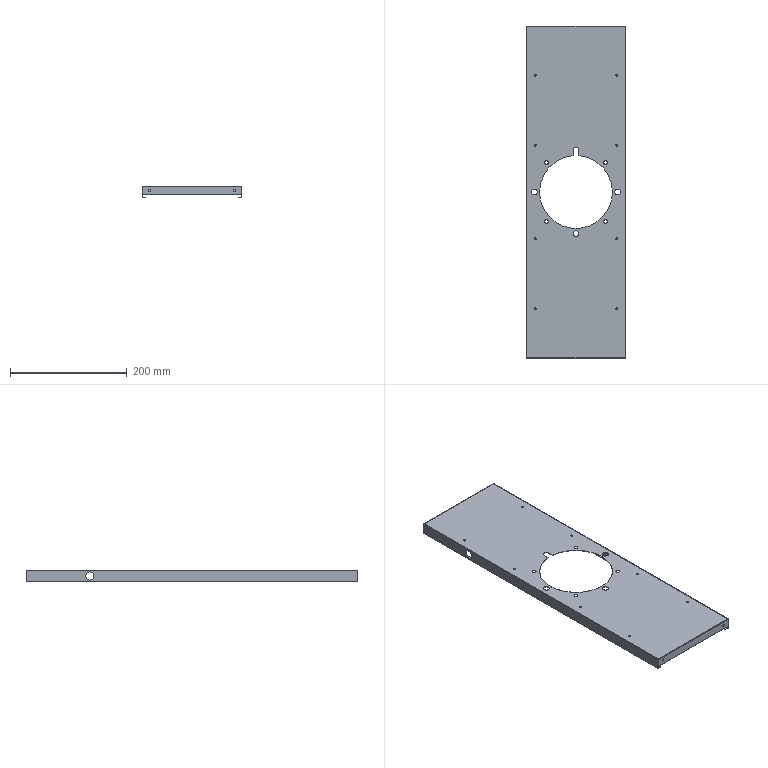Part | SolidWorks | features BaseBody 1 | 1 solid | 89 faces | box 170 x 568.8 x 20 mm | volume 69593 mm3 | cylinder 57 | plane 32 | commonest cylinder face diameters 3.5 x24 6.1 x8 10 x8 0.4 x6 1.6 x6 14 x4